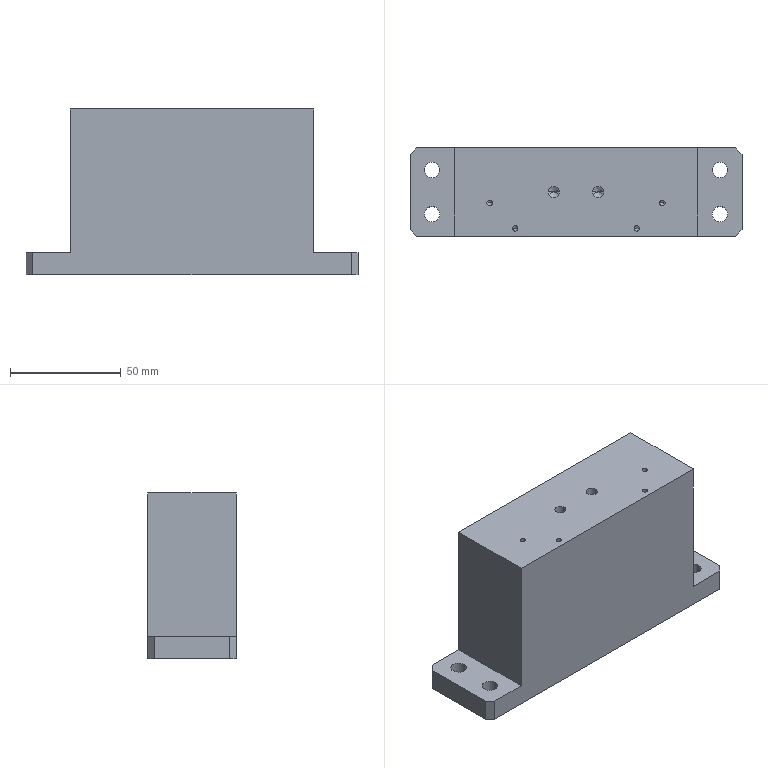Part | STEP file | 0217_207_Base | 1 solid | 46 faces | box 150 x 40 x 75 mm | volume 343539 mm3 | cylinder 20 | plane 14 | cone 12 | commonest cylinder face diameters 2.5 x8 7 x8 5 x4